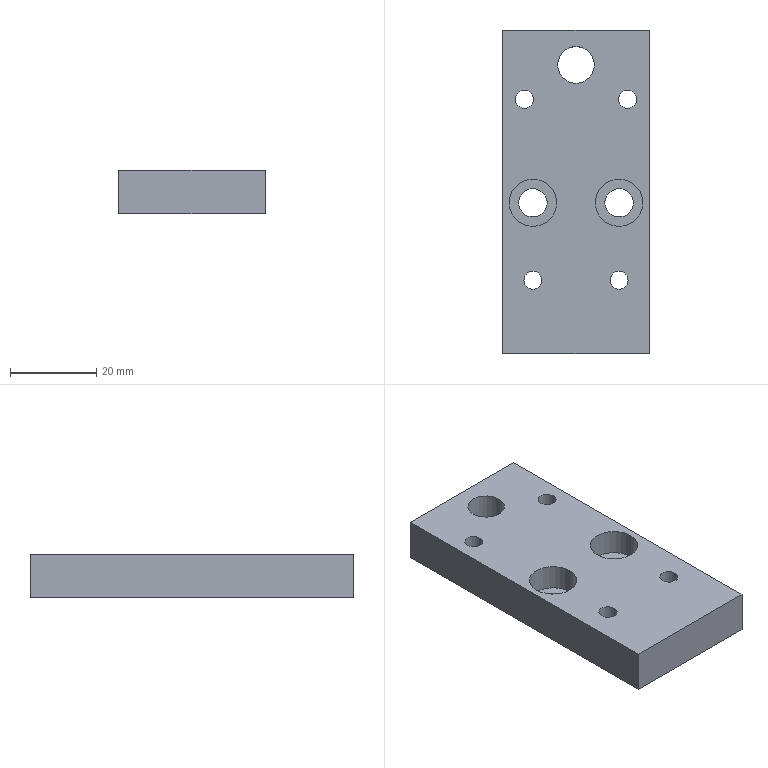Part | STEP file | push magnet slide seat spacer block | 1 solid | 26 faces | box 34 x 75 x 10 mm | volume 22964 mm3 | cylinder 18 | plane 8 | commonest cylinder face diameters 4.2 x8 6.6 x4 11 x4 8.5 x2